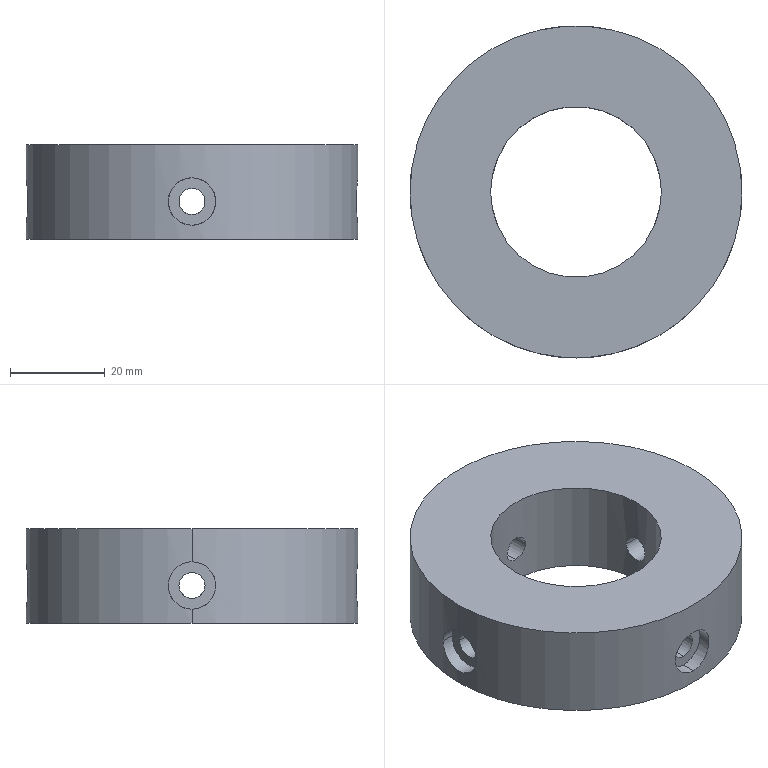Part | SolidWorks | features CirPattern 2, ICE 2, 3DProfileFeature 1, Extrusion 1, HoleWzd 1 | 1 solid | 42 faces | box 70 x 70 x 20 mm | volume 54005 mm3 | cylinder 28 | cone 8 | plane 6 | commonest cylinder face diameters 3.3 x8 5.5 x8 10 x8 36 x2 70 x2